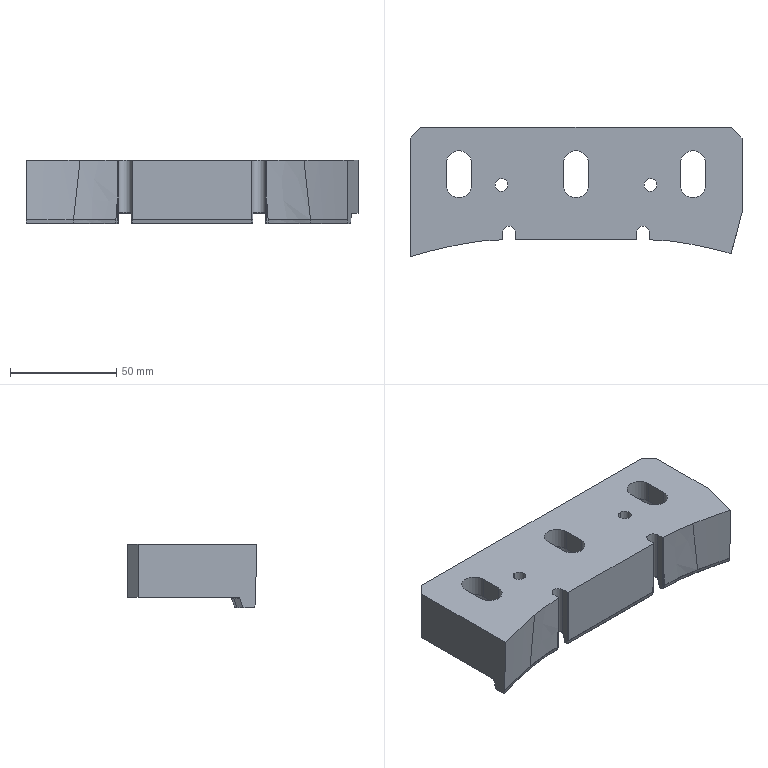NC program | Mastercam | posted with a generic post | part box 156 x 60.706 x 30 mm
Lines 37 to 876 of 78092:
N320 T20 M6
N330 G0 G90 G17 G54 X62.772 Y-53.181 A0. S1800 M3
N340 G43 H20 Z50.
N350 Z10.3
N360 G1 Z.3 F600.
N370 X65.011 Y-43.435 F3000.
N380 G3 X65.163 Y-42.092 I-5.848 J1.343
N390 X60.506 Y-36.244 I-6. J0.
N400 G1 X55.659 Y-35.177 Z.297
N410 X50.792 Y-34.2 Z.294
N420 X46.705 Y-33.514 Z.291
N430 X42.808 Y-33.035 Z.289
N440 X38.845 Y-32.722 Z.286
N450 X34.508 Y-32.572 Z.284
N460 X33.829 Y-32.53 Z.283
N470 X32.805 Y-32.365
N480 X31.804 Y-32.102 Z.282
N490 X31.554 Y-32.009
N500 X29.191 Y-32.575 Z.28
N510 X-29.159 Z.244
N520 X-31.568 Y-32.014 Z.243
N530 X-31.819 Y-32.107
N540 X-33.056 Y-32.43 Z.242
N550 X-34.262 Y-32.563 Z.241
N560 X-38.898 Y-32.725 Z.238
N570 X-42.806 Y-33.034 Z.236
N580 X-46.753 Y-33.521 Z.234
N590 X-50.791 Y-34.2 Z.231
N600 X-56.94 Y-35.45 Z.227
N610 X-63.058 Y-36.844 Z.223
N620 X-69.143 Y-38.378 Z.219
N630 X-75.19 Y-40.054 Z.216
N640 X-76.495 Y-40.34 Z.215
N650 X-77.826 Y-40.451 Z.214
N660 X-79.16 Y-40.386 Z.213
N670 X-80.474 Y-40.145 Z.212
N680 X-81.744 Y-39.733 Z.211
N690 X-82.949 Y-39.157
N700 X-84.068 Y-38.427 Z.21
N710 X-85.08 Y-37.556 Z.209
N720 X-85.968 Y-36.559 Z.208
N730 X-86.718 Y-35.453 Z.207
N740 X-87.314 Y-34.258 Z.206
N750 X-87.748 Y-32.995
N760 X-88.012 Y-31.686 Z.205
N770 X-88.1 Y-30.353 Z.204
N780 Y25.353 Z.17
N790 X-88.014 Y26.671 Z.169
N800 X-87.756 Y27.967 Z.168
N810 X-87.331 Y29.218 Z.167
N820 X-86.747 Y30.403 Z.166
N830 X-86.013 Y31.501
N840 X-85.142 Y32.495 Z.165
N850 X-80.142 Y37.495 Z.16
N860 X-79.148 Y38.366
N870 X-78.05 Y39.1 Z.159
N880 X-76.865 Y39.684 Z.158
N890 X-75.614 Y40.109 Z.157
N900 X-74.318 Y40.366 Z.156
N910 X-73. Y40.453
N920 X73. Z.066
N930 X74.318 Y40.366 Z.065
N940 X75.614 Y40.109 Z.064
N950 X76.865 Y39.684 Z.063
N960 X78.05 Y39.1 Z.062
N970 X79.148 Y38.366
N980 X80.142 Y37.495 Z.061
N990 X85.142 Y32.495 Z.056
N1000 X86.013 Y31.501
N1010 X86.747 Y30.403 Z.055
N1020 X87.331 Y29.218 Z.054
N1030 X87.756 Y27.967 Z.053
N1040 X88.014 Y26.671 Z.052
N1050 X88.1 Y25.353 Z.051
N1060 Y-11.111 Z.029
N1070 X82.628 Y-31.534 Z.016
N1080 X82.203 Y-32.786 Z.015
N1090 X81.618 Y-33.972 Z.014
N1100 X80.883 Y-35.071
N1110 X80.011 Y-36.065 Z.013
N1120 X79.016 Y-36.936 Z.012
N1130 X77.917 Y-37.67 Z.011
N1140 X76.731 Y-38.254 Z.01
N1150 X75.478 Y-38.678 Z.009
N1160 X74.181 Y-38.935
N1170 X72.862 Y-39.02 Z.008
N1180 X71.543 Y-38.932 Z.007
N1190 X70.247 Y-38.673 Z.006
N1200 X65.388 Y-37.413 Z.003
N1210 X60.506 Y-36.244 Z0.
N1220 X55.659 Y-35.177 Z-.003
N1230 X50.792 Y-34.2 Z-.006
N1240 X46.705 Y-33.514 Z-.009
N1250 X42.808 Y-33.035 Z-.011
N1260 X38.845 Y-32.722 Z-.014
N1270 X34.508 Y-32.572 Z-.016
N1280 X33.829 Y-32.53 Z-.017
N1290 X32.805 Y-32.365
N1300 X31.804 Y-32.102 Z-.018
N1310 X31.554 Y-32.009
N1320 X29.191 Y-32.575 Z-.02
N1330 X-29.159 Z-.056
N1340 X-31.568 Y-32.014 Z-.057
N1350 X-31.819 Y-32.107
N1360 X-33.056 Y-32.43 Z-.058
N1370 X-34.262 Y-32.563 Z-.059
N1380 X-38.898 Y-32.725 Z-.062
N1390 X-42.806 Y-33.034 Z-.064
N1400 X-46.753 Y-33.521 Z-.066
N1410 X-50.791 Y-34.2 Z-.069
N1420 X-56.94 Y-35.45 Z-.073
N1430 X-63.058 Y-36.844 Z-.077
N1440 X-69.143 Y-38.378 Z-.081
N1450 X-75.19 Y-40.054 Z-.084
N1460 X-76.495 Y-40.34 Z-.085
N1470 X-77.826 Y-40.451 Z-.086
N1480 X-79.16 Y-40.386 Z-.087
N1490 X-80.474 Y-40.145 Z-.088
N1500 X-81.744 Y-39.733 Z-.089
N1510 X-82.949 Y-39.157
N1520 X-84.068 Y-38.427 Z-.09
N1530 X-85.08 Y-37.556 Z-.091
N1540 X-85.968 Y-36.559 Z-.092
N1550 X-86.718 Y-35.453 Z-.093
N1560 X-87.314 Y-34.258 Z-.094
N1570 X-87.748 Y-32.995
N1580 X-88.012 Y-31.686 Z-.095
N1590 X-88.1 Y-30.353 Z-.096
N1600 Y25.353 Z-.13
N1610 X-88.014 Y26.671 Z-.131
N1620 X-87.756 Y27.967 Z-.132
N1630 X-87.331 Y29.218 Z-.133
N1640 X-86.747 Y30.403 Z-.134
N1650 X-86.013 Y31.501
N1660 X-85.142 Y32.495 Z-.135
N1670 X-80.142 Y37.495 Z-.14
N1680 X-79.148 Y38.366
N1690 X-78.05 Y39.1 Z-.141
N1700 X-76.865 Y39.684 Z-.142
N1710 X-75.614 Y40.109 Z-.143
N1720 X-74.318 Y40.366 Z-.144
N1730 X-73. Y40.453
N1740 X73. Z-.234
N1750 X74.318 Y40.366 Z-.235
N1760 X75.614 Y40.109 Z-.236
N1770 X76.865 Y39.684 Z-.237
N1780 X78.05 Y39.1 Z-.238
N1790 X79.148 Y38.366
N1800 X80.142 Y37.495 Z-.239
N1810 X85.142 Y32.495 Z-.244
N1820 X86.013 Y31.501
N1830 X86.747 Y30.403 Z-.245
N1840 X87.331 Y29.218 Z-.246
N1850 X87.756 Y27.967 Z-.247
N1860 X88.014 Y26.671 Z-.248
N1870 X88.1 Y25.353 Z-.249
N1880 Y-11.111 Z-.271
N1890 X82.628 Y-31.534 Z-.284
N1900 X82.203 Y-32.786 Z-.285
N1910 X81.618 Y-33.972 Z-.286
N1920 X80.883 Y-35.071
N1930 X80.011 Y-36.065 Z-.287
N1940 X79.016 Y-36.936 Z-.288
N1950 X77.917 Y-37.67 Z-.289
N1960 X76.731 Y-38.254 Z-.29
N1970 X75.478 Y-38.678 Z-.291
N1980 X74.181 Y-38.935
N1990 X72.862 Y-39.02 Z-.292
N2000 X71.543 Y-38.932 Z-.293
N2010 X70.247 Y-38.673 Z-.294
N2020 X65.388 Y-37.413 Z-.297
N2030 X60.506 Y-36.244 Z-.3
N2040 X55.659 Y-35.177 Z-.303
N2050 X50.792 Y-34.2 Z-.306
N2060 X46.705 Y-33.514 Z-.309
N2070 X42.808 Y-33.035 Z-.311
N2080 X38.845 Y-32.722 Z-.314
N2090 X34.508 Y-32.572 Z-.316
N2100 X33.829 Y-32.53 Z-.317
N2110 X32.805 Y-32.365
N2120 X31.804 Y-32.102 Z-.318
N2130 X31.554 Y-32.009
N2140 X29.191 Y-32.575 Z-.32
N2150 X-29.159 Z-.356
N2160 X-31.568 Y-32.014 Z-.357
N2170 X-31.819 Y-32.107
N2180 X-33.056 Y-32.43 Z-.358
N2190 X-34.262 Y-32.563 Z-.359
N2200 X-38.898 Y-32.725 Z-.362
N2210 X-42.806 Y-33.034 Z-.364
N2220 X-46.753 Y-33.521 Z-.366
N2230 X-50.791 Y-34.2 Z-.369
N2240 X-56.94 Y-35.45 Z-.373
N2250 X-63.058 Y-36.844 Z-.377
N2260 X-69.143 Y-38.378 Z-.381
N2270 X-75.19 Y-40.054 Z-.384
N2280 X-76.495 Y-40.34 Z-.385
N2290 X-77.826 Y-40.451 Z-.386
N2300 X-79.16 Y-40.386 Z-.387
N2310 X-80.474 Y-40.145 Z-.388
N2320 X-81.744 Y-39.733 Z-.389
N2330 X-82.949 Y-39.157
N2340 X-84.068 Y-38.427 Z-.39
N2350 X-85.08 Y-37.556 Z-.391
N2360 X-85.968 Y-36.559 Z-.392
N2370 X-86.718 Y-35.453 Z-.393
N2380 X-87.314 Y-34.258 Z-.394
N2390 X-87.748 Y-32.995
N2400 X-88.012 Y-31.686 Z-.395
N2410 X-88.1 Y-30.353 Z-.396
N2420 Y25.353 Z-.43
N2430 X-88.014 Y26.671 Z-.431
N2440 X-87.756 Y27.967 Z-.432
N2450 X-87.331 Y29.218 Z-.433
N2460 X-86.747 Y30.403 Z-.434
N2470 X-86.013 Y31.501
N2480 X-85.142 Y32.495 Z-.435
N2490 X-80.142 Y37.495 Z-.44
N2500 X-79.148 Y38.366
N2510 X-78.05 Y39.1 Z-.441
N2520 X-76.865 Y39.684 Z-.442
N2530 X-75.614 Y40.109 Z-.443
N2540 X-74.318 Y40.366 Z-.444
N2550 X-73. Y40.453
N2560 X73. Z-.534
N2570 X74.318 Y40.366 Z-.535
N2580 X75.614 Y40.109 Z-.536
N2590 X76.865 Y39.684 Z-.537
N2600 X78.05 Y39.1 Z-.538
N2610 X79.148 Y38.366
N2620 X80.142 Y37.495 Z-.539
N2630 X85.142 Y32.495 Z-.544
N2640 X86.013 Y31.501
N2650 X86.747 Y30.403 Z-.545
N2660 X87.331 Y29.218 Z-.546
N2670 X87.756 Y27.967 Z-.547
N2680 X88.014 Y26.671 Z-.548
N2690 X88.1 Y25.353 Z-.549
N2700 Y-11.111 Z-.571
N2710 X82.628 Y-31.534 Z-.584
N2720 X82.203 Y-32.786 Z-.585
N2730 X81.618 Y-33.972 Z-.586
N2740 X80.883 Y-35.071
N2750 X80.011 Y-36.065 Z-.587
N2760 X79.016 Y-36.936 Z-.588
N2770 X77.917 Y-37.67 Z-.589
N2780 X76.731 Y-38.254 Z-.59
N2790 X75.478 Y-38.678 Z-.591
N2800 X74.181 Y-38.935
N2810 X72.862 Y-39.02 Z-.592
N2820 X71.543 Y-38.932 Z-.593
N2830 X70.247 Y-38.673 Z-.594
N2840 X65.388 Y-37.413 Z-.597
N2850 X60.506 Y-36.244 Z-.6
N2860 X55.659 Y-35.177 Z-.603
N2870 X50.792 Y-34.2 Z-.606
N2880 X46.705 Y-33.514 Z-.609
N2890 X42.808 Y-33.035 Z-.611
N2900 X38.845 Y-32.722 Z-.614
N2910 X34.508 Y-32.572 Z-.616
N2920 X33.829 Y-32.53 Z-.617
N2930 X32.805 Y-32.365
N2940 X31.804 Y-32.102 Z-.618
N2950 X31.554 Y-32.009
N2960 X29.191 Y-32.575 Z-.62
N2970 X-29.159 Z-.656
N2980 X-31.568 Y-32.014 Z-.657
N2990 X-31.819 Y-32.107
N3000 X-33.056 Y-32.43 Z-.658
N3010 X-34.262 Y-32.563 Z-.659
N3020 X-38.898 Y-32.725 Z-.662
N3030 X-42.806 Y-33.034 Z-.664
N3040 X-46.753 Y-33.521 Z-.666
N3050 X-50.791 Y-34.2 Z-.669
N3060 X-56.94 Y-35.45 Z-.673
N3070 X-63.058 Y-36.844 Z-.677
N3080 X-69.143 Y-38.378 Z-.681
N3090 X-75.19 Y-40.054 Z-.684
N3100 X-76.495 Y-40.34 Z-.685
N3110 X-77.826 Y-40.451 Z-.686
N3120 X-79.16 Y-40.386 Z-.687
N3130 X-80.474 Y-40.145 Z-.688
N3140 X-81.744 Y-39.733 Z-.689
N3150 X-82.949 Y-39.157
N3160 X-84.068 Y-38.427 Z-.69
N3170 X-85.08 Y-37.556 Z-.691
N3180 X-85.968 Y-36.559 Z-.692
N3190 X-86.718 Y-35.453 Z-.693
N3200 X-87.314 Y-34.258 Z-.694
N3210 X-87.748 Y-32.995
N3220 X-88.012 Y-31.686 Z-.695
N3230 X-88.1 Y-30.353 Z-.696
N3240 Y25.353 Z-.73
N3250 X-88.014 Y26.671 Z-.731
N3260 X-87.756 Y27.967 Z-.732
N3270 X-87.331 Y29.218 Z-.733
N3280 X-86.747 Y30.403 Z-.734
N3290 X-86.013 Y31.501
N3300 X-85.142 Y32.495 Z-.735
N3310 X-80.142 Y37.495 Z-.74
N3320 X-79.148 Y38.366
N3330 X-78.05 Y39.1 Z-.741
N3340 X-76.865 Y39.684 Z-.742
N3350 X-75.614 Y40.109 Z-.743
N3360 X-74.318 Y40.366 Z-.744
N3370 X-73. Y40.453
N3380 X73. Z-.834
N3390 X74.318 Y40.366 Z-.835
N3400 X75.614 Y40.109 Z-.836
N3410 X76.865 Y39.684 Z-.837
N3420 X78.05 Y39.1 Z-.838
N3430 X79.148 Y38.366
N3440 X80.142 Y37.495 Z-.839
N3450 X85.142 Y32.495 Z-.844
N3460 X86.013 Y31.501
N3470 X86.747 Y30.403 Z-.845
N3480 X87.331 Y29.218 Z-.846
N3490 X87.756 Y27.967 Z-.847
N3500 X88.014 Y26.671 Z-.848
N3510 X88.1 Y25.353 Z-.849
N3520 Y-11.111 Z-.871
N3530 X82.628 Y-31.534 Z-.884
N3540 X82.203 Y-32.786 Z-.885
N3550 X81.618 Y-33.972 Z-.886
N3560 X80.883 Y-35.071
N3570 X80.011 Y-36.065 Z-.887
N3580 X79.016 Y-36.936 Z-.888
N3590 X77.917 Y-37.67 Z-.889
N3600 X76.731 Y-38.254 Z-.89
N3610 X75.478 Y-38.678 Z-.891
N3620 X74.181 Y-38.935
N3630 X72.862 Y-39.02 Z-.892
N3640 X71.543 Y-38.932 Z-.893
N3650 X70.247 Y-38.673 Z-.894
N3660 X65.388 Y-37.413 Z-.897
N3670 X60.506 Y-36.244 Z-.9
N3680 X55.659 Y-35.177 Z-.903
N3690 X50.792 Y-34.2 Z-.906
N3700 X46.705 Y-33.514 Z-.909
N3710 X42.808 Y-33.035 Z-.911
N3720 X38.845 Y-32.722 Z-.914
N3730 X34.508 Y-32.572 Z-.916
N3740 X33.829 Y-32.53 Z-.917
N3750 X32.805 Y-32.365
N3760 X31.804 Y-32.102 Z-.918
N3770 X31.554 Y-32.009
N3780 X29.191 Y-32.575 Z-.92
N3790 X-29.159 Z-.956
N3800 X-31.568 Y-32.014 Z-.957
N3810 X-31.819 Y-32.107
N3820 X-33.056 Y-32.43 Z-.958
N3830 X-34.262 Y-32.563 Z-.959
N3840 X-38.898 Y-32.725 Z-.962
N3850 X-42.806 Y-33.034 Z-.964
N3860 X-46.753 Y-33.521 Z-.966
N3870 X-50.791 Y-34.2 Z-.969
N3880 X-56.94 Y-35.45 Z-.973
N3890 X-63.058 Y-36.844 Z-.977
N3900 X-69.143 Y-38.378 Z-.981
N3910 X-75.19 Y-40.054 Z-.984
N3920 X-76.495 Y-40.34 Z-.985
N3930 X-77.826 Y-40.451 Z-.986
N3940 X-79.16 Y-40.386 Z-.987
N3950 X-80.474 Y-40.145 Z-.988
N3960 X-81.744 Y-39.733 Z-.989
N3970 X-82.949 Y-39.157
N3980 X-84.068 Y-38.427 Z-.99
N3990 X-85.08 Y-37.556 Z-.991
N4000 X-85.968 Y-36.559 Z-.992
N4010 X-86.718 Y-35.453 Z-.993
N4020 X-87.314 Y-34.258 Z-.994
N4030 X-87.748 Y-32.995
N4040 X-88.012 Y-31.686 Z-.995
N4050 X-88.1 Y-30.353 Z-.996
N4060 Y25.353 Z-1.03
N4070 X-88.014 Y26.671 Z-1.031
N4080 X-87.756 Y27.967 Z-1.032
N4090 X-87.331 Y29.218 Z-1.033
N4100 X-86.747 Y30.403 Z-1.034
N4110 X-86.013 Y31.501
N4120 X-85.142 Y32.495 Z-1.035
N4130 X-80.142 Y37.495 Z-1.04
N4140 X-79.148 Y38.366
N4150 X-78.05 Y39.1 Z-1.041
N4160 X-76.865 Y39.684 Z-1.042
N4170 X-75.614 Y40.109 Z-1.043
N4180 X-74.318 Y40.366 Z-1.044
N4190 X-73. Y40.453
N4200 X73. Z-1.134
N4210 X74.318 Y40.366 Z-1.135
N4220 X75.614 Y40.109 Z-1.136
N4230 X76.865 Y39.684 Z-1.137
N4240 X78.05 Y39.1 Z-1.138
N4250 X79.148 Y38.366
N4260 X80.142 Y37.495 Z-1.139
N4270 X85.142 Y32.495 Z-1.144
N4280 X86.013 Y31.501
N4290 X86.747 Y30.403 Z-1.145
N4300 X87.331 Y29.218 Z-1.146
N4310 X87.756 Y27.967 Z-1.147
N4320 X88.014 Y26.671 Z-1.148
N4330 X88.1 Y25.353 Z-1.149
N4340 Y-11.111 Z-1.171
N4350 X82.628 Y-31.534 Z-1.184
N4360 X82.203 Y-32.786 Z-1.185
N4370 X81.618 Y-33.972 Z-1.186
N4380 X80.883 Y-35.071
N4390 X80.011 Y-36.065 Z-1.187
N4400 X79.016 Y-36.936 Z-1.188
N4410 X77.917 Y-37.67 Z-1.189
N4420 X76.731 Y-38.254 Z-1.19
N4430 X75.478 Y-38.678 Z-1.191
N4440 X74.181 Y-38.935
N4450 X72.862 Y-39.02 Z-1.192
N4460 X71.543 Y-38.932 Z-1.193
N4470 X70.247 Y-38.673 Z-1.194
N4480 X65.388 Y-37.413 Z-1.197
N4490 X60.506 Y-36.244 Z-1.2
N4500 X55.659 Y-35.177 Z-1.203
N4510 X50.792 Y-34.2 Z-1.206
N4520 X46.705 Y-33.514 Z-1.209
N4530 X42.808 Y-33.035 Z-1.211
N4540 X38.845 Y-32.722 Z-1.214
N4550 X34.508 Y-32.572 Z-1.216
N4560 X33.829 Y-32.53 Z-1.217
N4570 X32.805 Y-32.365
N4580 X31.804 Y-32.102 Z-1.218
N4590 X31.554 Y-32.009
N4600 X29.191 Y-32.575 Z-1.22
N4610 X-29.159 Z-1.256
N4620 X-31.568 Y-32.014 Z-1.257
N4630 X-31.819 Y-32.107
N4640 X-33.056 Y-32.43 Z-1.258
N4650 X-34.262 Y-32.563 Z-1.259
N4660 X-38.898 Y-32.725 Z-1.262
N4670 X-42.806 Y-33.034 Z-1.264
N4680 X-46.753 Y-33.521 Z-1.266
N4690 X-50.791 Y-34.2 Z-1.269
N4700 X-56.94 Y-35.45 Z-1.273
N4710 X-63.058 Y-36.844 Z-1.277
N4720 X-69.143 Y-38.378 Z-1.281
N4730 X-75.19 Y-40.054 Z-1.284
N4740 X-76.495 Y-40.34 Z-1.285
N4750 X-77.826 Y-40.451 Z-1.286
N4760 X-79.16 Y-40.386 Z-1.287
N4770 X-80.474 Y-40.145 Z-1.288
N4780 X-81.744 Y-39.733 Z-1.289
N4790 X-82.949 Y-39.157
N4800 X-84.068 Y-38.427 Z-1.29
N4810 X-85.08 Y-37.556 Z-1.291
N4820 X-85.968 Y-36.559 Z-1.292
N4830 X-86.718 Y-35.453 Z-1.293
N4840 X-87.314 Y-34.258 Z-1.294
N4850 X-87.748 Y-32.995
N4860 X-88.012 Y-31.686 Z-1.295
N4870 X-88.1 Y-30.353 Z-1.296
N4880 Y25.353 Z-1.33
N4890 X-88.014 Y26.671 Z-1.331
N4900 X-87.756 Y27.967 Z-1.332
N4910 X-87.331 Y29.218 Z-1.333
N4920 X-86.747 Y30.403 Z-1.334
N4930 X-86.013 Y31.501
N4940 X-85.142 Y32.495 Z-1.335
N4950 X-80.142 Y37.495 Z-1.34
N4960 X-79.148 Y38.366
N4970 X-78.05 Y39.1 Z-1.341
N4980 X-76.865 Y39.684 Z-1.342
N4990 X-75.614 Y40.109 Z-1.343
N5000 X-74.318 Y40.366 Z-1.344
N5010 X-73. Y40.453
N5020 X73. Z-1.434
N5030 X74.318 Y40.366 Z-1.435
N5040 X75.614 Y40.109 Z-1.436
N5050 X76.865 Y39.684 Z-1.437
N5060 X78.05 Y39.1 Z-1.438
N5070 X79.148 Y38.366
N5080 X80.142 Y37.495 Z-1.439
N5090 X85.142 Y32.495 Z-1.444
N5100 X86.013 Y31.501
N5110 X86.747 Y30.403 Z-1.445
N5120 X87.331 Y29.218 Z-1.446
N5130 X87.756 Y27.967 Z-1.447
N5140 X88.014 Y26.671 Z-1.448
N5150 X88.1 Y25.353 Z-1.449
N5160 Y-11.111 Z-1.471
N5170 X82.628 Y-31.534 Z-1.484
N5180 X82.203 Y-32.786 Z-1.485
N5190 X81.618 Y-33.972 Z-1.486
N5200 X80.883 Y-35.071
N5210 X80.011 Y-36.065 Z-1.487
N5220 X79.016 Y-36.936 Z-1.488
N5230 X77.917 Y-37.67 Z-1.489
N5240 X76.731 Y-38.254 Z-1.49
N5250 X75.478 Y-38.678 Z-1.491
N5260 X74.181 Y-38.935
N5270 X72.862 Y-39.02 Z-1.492
N5280 X71.543 Y-38.932 Z-1.493
N5290 X70.247 Y-38.673 Z-1.494
N5300 X65.388 Y-37.413 Z-1.497
N5310 X60.506 Y-36.244 Z-1.5
N5320 X55.659 Y-35.177 Z-1.503
N5330 X50.792 Y-34.2 Z-1.506
N5340 X46.705 Y-33.514 Z-1.509
N5350 X42.808 Y-33.035 Z-1.511
N5360 X38.845 Y-32.722 Z-1.514
N5370 X34.508 Y-32.572 Z-1.516
N5380 X33.829 Y-32.53 Z-1.517
N5390 X32.805 Y-32.365
N5400 X31.804 Y-32.102 Z-1.518
N5410 X31.554 Y-32.009
N5420 X29.191 Y-32.575 Z-1.52
N5430 X-29.159 Z-1.556
N5440 X-31.568 Y-32.014 Z-1.557
N5450 X-31.819 Y-32.107
N5460 X-33.056 Y-32.43 Z-1.558
N5470 X-34.262 Y-32.563 Z-1.559
N5480 X-38.898 Y-32.725 Z-1.562
N5490 X-42.806 Y-33.034 Z-1.564
N5500 X-46.753 Y-33.521 Z-1.566
N5510 X-50.791 Y-34.2 Z-1.569
N5520 X-56.94 Y-35.45 Z-1.573
N5530 X-63.058 Y-36.844 Z-1.577
N5540 X-69.143 Y-38.378 Z-1.581
N5550 X-75.19 Y-40.054 Z-1.584
N5560 X-76.495 Y-40.34 Z-1.585
N5570 X-77.826 Y-40.451 Z-1.586
N5580 X-79.16 Y-40.386 Z-1.587
N5590 X-80.474 Y-40.145 Z-1.588
N5600 X-81.744 Y-39.733 Z-1.589
N5610 X-82.949 Y-39.157
N5620 X-84.068 Y-38.427 Z-1.59
N5630 X-85.08 Y-37.556 Z-1.591
N5640 X-85.968 Y-36.559 Z-1.592
N5650 X-86.718 Y-35.453 Z-1.593
N5660 X-87.314 Y-34.258 Z-1.594
N5670 X-87.748 Y-32.995
N5680 X-88.012 Y-31.686 Z-1.595
N5690 X-88.1 Y-30.353 Z-1.596
N5700 Y25.353 Z-1.63
N5710 X-88.014 Y26.671 Z-1.631
N5720 X-87.756 Y27.967 Z-1.632
N5730 X-87.331 Y29.218 Z-1.633
N5740 X-86.747 Y30.403 Z-1.634
N5750 X-86.013 Y31.501
N5760 X-85.142 Y32.495 Z-1.635
N5770 X-80.142 Y37.495 Z-1.64
N5780 X-79.148 Y38.366
N5790 X-78.05 Y39.1 Z-1.641
N5800 X-76.865 Y39.684 Z-1.642
N5810 X-75.614 Y40.109 Z-1.643
N5820 X-74.318 Y40.366 Z-1.644
N5830 X-73. Y40.453
N5840 X73. Z-1.734
N5850 X74.318 Y40.366 Z-1.735
N5860 X75.614 Y40.109 Z-1.736
N5870 X76.865 Y39.684 Z-1.737
N5880 X78.05 Y39.1 Z-1.738
N5890 X79.148 Y38.366
N5900 X80.142 Y37.495 Z-1.739
N5910 X85.142 Y32.495 Z-1.744
N5920 X86.013 Y31.501
N5930 X86.747 Y30.403 Z-1.745
N5940 X87.331 Y29.218 Z-1.746
N5950 X87.756 Y27.967 Z-1.747
N5960 X88.014 Y26.671 Z-1.748
N5970 X88.1 Y25.353 Z-1.749
N5980 Y-11.111 Z-1.771
N5990 X82.628 Y-31.534 Z-1.784
N6000 X82.203 Y-32.786 Z-1.785
N6010 X81.618 Y-33.972 Z-1.786
N6020 X80.883 Y-35.071
N6030 X80.011 Y-36.065 Z-1.787
N6040 X79.016 Y-36.936 Z-1.788
N6050 X77.917 Y-37.67 Z-1.789
N6060 X76.731 Y-38.254 Z-1.79
N6070 X75.478 Y-38.678 Z-1.791
N6080 X74.181 Y-38.935
N6090 X72.862 Y-39.02 Z-1.792
N6100 X71.543 Y-38.932 Z-1.793
N6110 X70.247 Y-38.673 Z-1.794
N6120 X65.388 Y-37.413 Z-1.797
N6130 X60.506 Y-36.244 Z-1.8
N6140 X55.659 Y-35.177 Z-1.803
N6150 X50.792 Y-34.2 Z-1.806
N6160 X46.705 Y-33.514 Z-1.809
N6170 X42.808 Y-33.035 Z-1.811
N6180 X38.845 Y-32.722 Z-1.814
N6190 X34.508 Y-32.572 Z-1.816
N6200 X33.829 Y-32.53 Z-1.817
N6210 X32.805 Y-32.365
N6220 X31.804 Y-32.102 Z-1.818
N6230 X31.554 Y-32.009
N6240 X29.191 Y-32.575 Z-1.82
N6250 X-29.159 Z-1.856
N6260 X-31.568 Y-32.014 Z-1.857
N6270 X-31.819 Y-32.107
N6280 X-33.056 Y-32.43 Z-1.858
N6290 X-34.262 Y-32.563 Z-1.859
N6300 X-38.898 Y-32.725 Z-1.862
N6310 X-42.806 Y-33.034 Z-1.864
N6320 X-46.753 Y-33.521 Z-1.866
N6330 X-50.791 Y-34.2 Z-1.869
N6340 X-56.94 Y-35.45 Z-1.873
N6350 X-63.058 Y-36.844 Z-1.877
N6360 X-69.143 Y-38.378 Z-1.881
N6370 X-75.19 Y-40.054 Z-1.884
N6380 X-76.495 Y-40.34 Z-1.885
N6390 X-77.826 Y-40.451 Z-1.886
N6400 X-79.16 Y-40.386 Z-1.887
N6410 X-80.474 Y-40.145 Z-1.888
N6420 X-81.744 Y-39.733 Z-1.889
N6430 X-82.949 Y-39.157
N6440 X-84.068 Y-38.427 Z-1.89
N6450 X-85.08 Y-37.556 Z-1.891
N6460 X-85.968 Y-36.559 Z-1.892
N6470 X-86.718 Y-35.453 Z-1.893
N6480 X-87.314 Y-34.258 Z-1.894
N6490 X-87.748 Y-32.995
N6500 X-88.012 Y-31.686 Z-1.895
N6510 X-88.1 Y-30.353 Z-1.896
N6520 Y25.353 Z-1.93
N6530 X-88.014 Y26.671 Z-1.931
N6540 X-87.756 Y27.967 Z-1.932
N6550 X-87.331 Y29.218 Z-1.933
N6560 X-86.747 Y30.403 Z-1.934
N6570 X-86.013 Y31.501
N6580 X-85.142 Y32.495 Z-1.935
N6590 X-80.142 Y37.495 Z-1.94
N6600 X-79.148 Y38.366
N6610 X-78.05 Y39.1 Z-1.941
N6620 X-76.865 Y39.684 Z-1.942
N6630 X-75.614 Y40.109 Z-1.943
N6640 X-74.318 Y40.366 Z-1.944
N6650 X-73. Y40.453
N6660 X73. Z-2.034
N6670 X74.318 Y40.366 Z-2.035
N6680 X75.614 Y40.109 Z-2.036
N6690 X76.865 Y39.684 Z-2.037
N6700 X78.05 Y39.1 Z-2.038
N6710 X79.148 Y38.366
N6720 X80.142 Y37.495 Z-2.039
N6730 X85.142 Y32.495 Z-2.044
N6740 X86.013 Y31.501
N6750 X86.747 Y30.403 Z-2.045
N6760 X87.331 Y29.218 Z-2.046
N6770 X87.756 Y27.967 Z-2.047
N6780 X88.014 Y26.671 Z-2.048
N6790 X88.1 Y25.353 Z-2.049
N6800 Y-11.111 Z-2.071
N6810 X82.628 Y-31.534 Z-2.084
N6820 X82.203 Y-32.786 Z-2.085
N6830 X81.618 Y-33.972 Z-2.086
N6840 X80.883 Y-35.071
N6850 X80.011 Y-36.065 Z-2.087
N6860 X79.016 Y-36.936 Z-2.088
N6870 X77.917 Y-37.67 Z-2.089
N6880 X76.731 Y-38.254 Z-2.09
N6890 X75.478 Y-38.678 Z-2.091
N6900 X74.181 Y-38.935
N6910 X72.862 Y-39.02 Z-2.092
N6920 X71.543 Y-38.932 Z-2.093
N6930 X70.247 Y-38.673 Z-2.094
N6940 X65.388 Y-37.413 Z-2.097
N6950 X60.506 Y-36.244 Z-2.1
N6960 X55.659 Y-35.177 Z-2.103
N6970 X50.792 Y-34.2 Z-2.106
N6980 X46.705 Y-33.514 Z-2.109
N6990 X42.808 Y-33.035 Z-2.111
N7000 X38.845 Y-32.722 Z-2.114
N7010 X34.508 Y-32.572 Z-2.116
N7020 X33.829 Y-32.53 Z-2.117
N7030 X32.805 Y-32.365
N7040 X31.804 Y-32.102 Z-2.118
N7050 X31.554 Y-32.009
N7060 X29.191 Y-32.575 Z-2.12
N7070 X-29.159 Z-2.156
N7080 X-31.568 Y-32.014 Z-2.157
N7090 X-31.819 Y-32.107
N7100 X-33.056 Y-32.43 Z-2.158
N7110 X-34.262 Y-32.563 Z-2.159
N7120 X-38.898 Y-32.725 Z-2.162
N7130 X-42.806 Y-33.034 Z-2.164
N7140 X-46.753 Y-33.521 Z-2.166
N7150 X-50.791 Y-34.2 Z-2.169
N7160 X-56.94 Y-35.45 Z-2.173
N7170 X-63.058 Y-36.844 Z-2.177
N7180 X-69.143 Y-38.378 Z-2.181
N7190 X-75.19 Y-40.054 Z-2.184
N7200 X-76.495 Y-40.34 Z-2.185
N7210 X-77.826 Y-40.451 Z-2.186
N7220 X-79.16 Y-40.386 Z-2.187
N7230 X-80.474 Y-40.145 Z-2.188
N7240 X-81.744 Y-39.733 Z-2.189
N7250 X-82.949 Y-39.157
N7260 X-84.068 Y-38.427 Z-2.19
N7270 X-85.08 Y-37.556 Z-2.191
N7280 X-85.968 Y-36.559 Z-2.192
N7290 X-86.718 Y-35.453 Z-2.193
N7300 X-87.314 Y-34.258 Z-2.194
N7310 X-87.748 Y-32.995
N7320 X-88.012 Y-31.686 Z-2.195
N7330 X-88.1 Y-30.353 Z-2.196
N7340 Y25.353 Z-2.23
N7350 X-88.014 Y26.671 Z-2.231
N7360 X-87.756 Y27.967 Z-2.232
N7370 X-87.331 Y29.218 Z-2.233
N7380 X-86.747 Y30.403 Z-2.234
N7390 X-86.013 Y31.501
N7400 X-85.142 Y32.495 Z-2.235
N7410 X-80.142 Y37.495 Z-2.24
N7420 X-79.148 Y38.366
N7430 X-78.05 Y39.1 Z-2.241
N7440 X-76.865 Y39.684 Z-2.242
N7450 X-75.614 Y40.109 Z-2.243
N7460 X-74.318 Y40.366 Z-2.244
N7470 X-73. Y40.453
N7480 X73. Z-2.334
N7490 X74.318 Y40.366 Z-2.335
N7500 X75.614 Y40.109 Z-2.336
N7510 X76.865 Y39.684 Z-2.337
N7520 X78.05 Y39.1 Z-2.338
N7530 X79.148 Y38.366
N7540 X80.142 Y37.495 Z-2.339
N7550 X85.142 Y32.495 Z-2.344
N7560 X86.013 Y31.501
N7570 X86.747 Y30.403 Z-2.345
N7580 X87.331 Y29.218 Z-2.346
N7590 X87.756 Y27.967 Z-2.347
N7600 X88.014 Y26.671 Z-2.348
N7610 X88.1 Y25.353 Z-2.349
N7620 Y-11.111 Z-2.371
N7630 X82.628 Y-31.534 Z-2.384
N7640 X82.203 Y-32.786 Z-2.385
N7650 X81.618 Y-33.972 Z-2.386
N7660 X80.883 Y-35.071
N7670 X80.011 Y-36.065 Z-2.387
N7680 X79.016 Y-36.936 Z-2.388
N7690 X77.917 Y-37.67 Z-2.389
N7700 X76.731 Y-38.254 Z-2.39
N7710 X75.478 Y-38.678 Z-2.391
N7720 X74.181 Y-38.935
N7730 X72.862 Y-39.02 Z-2.392
N7740 X71.543 Y-38.932 Z-2.393
N7750 X70.247 Y-38.673 Z-2.394
N7760 X65.388 Y-37.413 Z-2.397
N7770 X60.506 Y-36.244 Z-2.4
N7780 X55.659 Y-35.177 Z-2.403
N7790 X50.792 Y-34.2 Z-2.406
N7800 X46.705 Y-33.514 Z-2.409
N7810 X42.808 Y-33.035 Z-2.411
N7820 X38.845 Y-32.722 Z-2.414
N7830 X34.508 Y-32.572 Z-2.416
N7840 X33.829 Y-32.53 Z-2.417
N7850 X32.805 Y-32.365
N7860 X31.804 Y-32.102 Z-2.418
N7870 X31.554 Y-32.009
N7880 X29.191 Y-32.575 Z-2.42
N7890 X-29.159 Z-2.456
N7900 X-31.568 Y-32.014 Z-2.457
N7910 X-31.819 Y-32.107
N7920 X-33.056 Y-32.43 Z-2.458
N7930 X-34.262 Y-32.563 Z-2.459
N7940 X-38.898 Y-32.725 Z-2.462
N7950 X-42.806 Y-33.034 Z-2.464
N7960 X-46.753 Y-33.521 Z-2.466
N7970 X-50.791 Y-34.2 Z-2.469
N7980 X-56.94 Y-35.45 Z-2.473
N7990 X-63.058 Y-36.844 Z-2.477
N8000 X-69.143 Y-38.378 Z-2.481
N8010 X-75.19 Y-40.054 Z-2.484
N8020 X-76.495 Y-40.34 Z-2.485
N8030 X-77.826 Y-40.451 Z-2.486
N8040 X-79.16 Y-40.386 Z-2.487
N8050 X-80.474 Y-40.145 Z-2.488
N8060 X-81.744 Y-39.733 Z-2.489
N8070 X-82.949 Y-39.157
N8080 X-84.068 Y-38.427 Z-2.49
N8090 X-85.08 Y-37.556 Z-2.491
N8100 X-85.968 Y-36.559 Z-2.492
N8110 X-86.718 Y-35.453 Z-2.493
N8120 X-87.314 Y-34.258 Z-2.494
N8130 X-87.748 Y-32.995
N8140 X-88.012 Y-31.686 Z-2.495
N8150 X-88.1 Y-30.353 Z-2.496
N8160 Y25.353 Z-2.53
N8170 X-88.014 Y26.671 Z-2.531
N8180 X-87.756 Y27.967 Z-2.532
N8190 X-87.331 Y29.218 Z-2.533
N8200 X-86.747 Y30.403 Z-2.534
N8210 X-86.013 Y31.501
N8220 X-85.142 Y32.495 Z-2.535
N8230 X-80.142 Y37.495 Z-2.54
N8240 X-79.148 Y38.366
N8250 X-78.05 Y39.1 Z-2.541
N8260 X-76.865 Y39.684 Z-2.542
N8270 X-75.614 Y40.109 Z-2.543
N8280 X-74.318 Y40.366 Z-2.544
N8290 X-73. Y40.453
N8300 X73. Z-2.634
N8310 X74.318 Y40.366 Z-2.635
N8320 X75.614 Y40.109 Z-2.636
N8330 X76.865 Y39.684 Z-2.637
N8340 X78.05 Y39.1 Z-2.638
N8350 X79.148 Y38.366
N8360 X80.142 Y37.495 Z-2.639
N8370 X85.142 Y32.495 Z-2.644
N8380 X86.013 Y31.501
N8390 X86.747 Y30.403 Z-2.645
N8400 X87.331 Y29.218 Z-2.646
N8410 X87.756 Y27.967 Z-2.647
N8420 X88.014 Y26.671 Z-2.648
N8430 X88.1 Y25.353 Z-2.649
N8440 Y-11.111 Z-2.671
N8450 X82.628 Y-31.534 Z-2.684
N8460 X82.203 Y-32.786 Z-2.685
N8470 X81.618 Y-33.972 Z-2.686
N8480 X80.883 Y-35.071
N8490 X80.011 Y-36.065 Z-2.687
N8500 X79.016 Y-36.936 Z-2.688
N8510 X77.917 Y-37.67 Z-2.689
N8520 X76.731 Y-38.254 Z-2.69
N8530 X75.478 Y-38.678 Z-2.691
N8540 X74.181 Y-38.935
N8550 X72.862 Y-39.02 Z-2.692
N8560 X71.543 Y-38.932 Z-2.693
N8570 X70.247 Y-38.673 Z-2.694
N8580 X65.388 Y-37.413 Z-2.697
N8590 X60.506 Y-36.244 Z-2.7
N8600 X55.659 Y-35.177 Z-2.703
N8610 X50.792 Y-34.2 Z-2.706
N8620 X46.705 Y-33.514 Z-2.709
N8630 X42.808 Y-33.035 Z-2.711
N8640 X38.845 Y-32.722 Z-2.714
N8650 X34.508 Y-32.572 Z-2.716
N8660 X33.829 Y-32.53 Z-2.717
N8670 X32.805 Y-32.365
N8680 X31.804 Y-32.102 Z-2.718
N8690 X31.554 Y-32.009
N8700 X29.191 Y-32.575 Z-2.72
N8710 X-29.159 Z-2.756